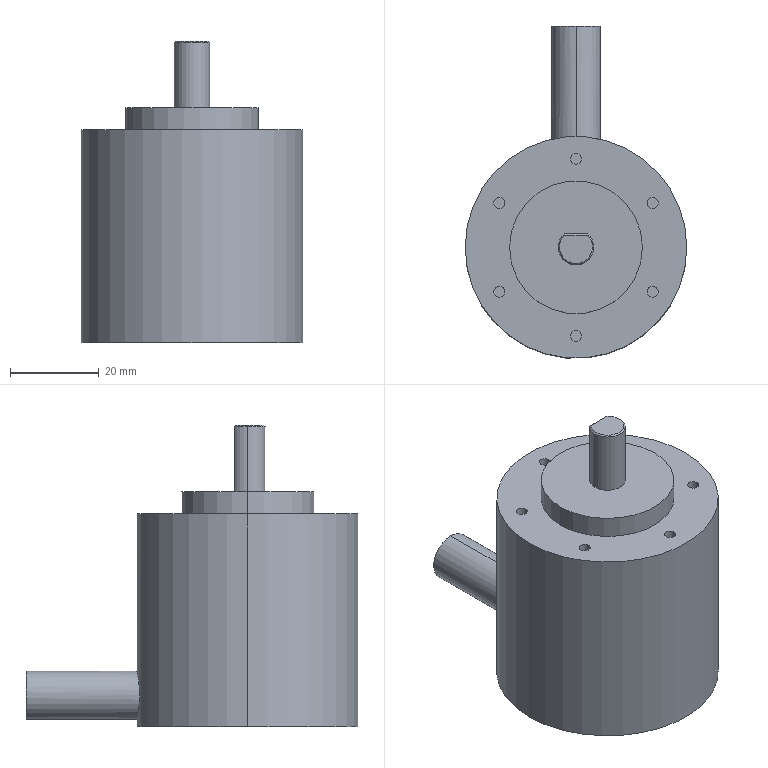Part | SolidWorks | features ICE 4, Chamfer 1, Extrusion 1 | 1 solid | 37 faces | box 50 x 75 x 68 mm | volume 100645 mm3 | cylinder 21 | plane 13 | cone 3 | commonest cylinder face diameters 2.5 x12 8 x3 10.956 x2 30 x2 50 x2
STEP:
#1=CARTESIAN_POINT('',(-1.25,20.,41.));
#2=VERTEX_POINT('',#1);
#3=CARTESIAN_POINT('',(1.25,20.,41.));
#4=VERTEX_POINT('',#3);
#5=CARTESIAN_POINT('',(0.,20.,41.));
#6=DIRECTION('',(0.,0.,1.));
#7=DIRECTION('',(1.,0.,0.));
#8=AXIS2_PLACEMENT_3D('',#5,#6,#7);
#9=CIRCLE('',#8,1.25);
#10=EDGE_CURVE('',#2,#4,#9,.T.);
#11=ORIENTED_EDGE('',*,*,#10,.F.);
#12=CARTESIAN_POINT('',(-1.25,20.,48.));
#13=VERTEX_POINT('',#12);
#14=CARTESIAN_POINT('',(-1.25,20.,41.));
#15=DIRECTION('',(0.,0.,1.));
#16=VECTOR('',#15,1000.);
#17=LINE('',#14,#16);
#18=EDGE_CURVE('',#2,#13,#17,.T.);
#19=ORIENTED_EDGE('',*,*,#18,.T.);
#20=CARTESIAN_POINT('',(1.25,20.,48.));
#21=VERTEX_POINT('',#20);
#22=CARTESIAN_POINT('',(0.,20.,48.));
#23=DIRECTION('',(0.,0.,1.));
#24=DIRECTION('',(1.,0.,0.));
#25=AXIS2_PLACEMENT_3D('',#22,#23,#24);
#26=CIRCLE('',#25,1.25);
#27=EDGE_CURVE('',#13,#21,#26,.T.);
#28=ORIENTED_EDGE('',*,*,#27,.T.);
#29=CARTESIAN_POINT('',(1.25,20.,41.));
#30=DIRECTION('',(0.,0.,1.));
#31=VECTOR('',#30,1000.);
#32=LINE('',#29,#31);
#33=EDGE_CURVE('',#4,#21,#32,.T.);
#34=ORIENTED_EDGE('',*,*,#33,.F.);
#35=EDGE_LOOP('',(#11,#19,#28,#34));
#36=FACE_OUTER_BOUND('',#35,.T.);
#37=CARTESIAN_POINT('',(0.,20.,41.));
#38=DIRECTION('',(0.,0.,1.));
#39=DIRECTION('',(1.,0.,0.));
#40=AXIS2_PLACEMENT_3D('',#37,#38,#39);
#41=CYLINDRICAL_SURFACE('',#40,1.25);
#42=ADVANCED_FACE('',(#36),#41,.F.);
#43=CARTESIAN_POINT('',(-18.571,10.,41.));
#44=VERTEX_POINT('',#43);
#45=CARTESIAN_POINT('',(-16.071,10.,41.));
#46=VERTEX_POINT('',#45);
#47=CARTESIAN_POINT('',(-17.321,10.,41.));
#48=DIRECTION('',(0.,0.,1.));
#49=DIRECTION('',(1.,0.,0.));
#50=AXIS2_PLACEMENT_3D('',#47,#48,#49);
#51=CIRCLE('',#50,1.25);
#52=EDGE_CURVE('',#44,#46,#51,.T.);
#53=ORIENTED_EDGE('',*,*,#52,.F.);
#54=CARTESIAN_POINT('',(-18.571,10.,48.));
#55=VERTEX_POINT('',#54);
#56=CARTESIAN_POINT('',(-18.571,10.,41.));
#57=DIRECTION('',(0.,0.,1.));
#58=VECTOR('',#57,1000.);
#59=LINE('',#56,#58);
#60=EDGE_CURVE('',#44,#55,#59,.T.);
#61=ORIENTED_EDGE('',*,*,#60,.T.);
#62=CARTESIAN_POINT('',(-16.071,10.,48.));
#63=VERTEX_POINT('',#62);
#64=CARTESIAN_POINT('',(-17.321,10.,48.));
#65=DIRECTION('',(0.,0.,1.));
#66=DIRECTION('',(1.,0.,0.));
#67=AXIS2_PLACEMENT_3D('',#64,#65,#66);
#68=CIRCLE('',#67,1.25);
#69=EDGE_CURVE('',#55,#63,#68,.T.);
#70=ORIENTED_EDGE('',*,*,#69,.T.);
#71=CARTESIAN_POINT('',(-16.071,10.,41.));
#72=DIRECTION('',(0.,0.,1.));
#73=VECTOR('',#72,1000.);
#74=LINE('',#71,#73);
#75=EDGE_CURVE('',#46,#63,#74,.T.);
#76=ORIENTED_EDGE('',*,*,#75,.F.);
#77=EDGE_LOOP('',(#53,#61,#70,#76));
#78=FACE_OUTER_BOUND('',#77,.T.);
#79=CARTESIAN_POINT('',(-17.321,10.,41.));
#80=DIRECTION('',(0.,0.,1.));
#81=DIRECTION('',(1.,0.,0.));
#82=AXIS2_PLACEMENT_3D('',#79,#80,#81);
#83=CYLINDRICAL_SURFACE('',#82,1.25);
#84=ADVANCED_FACE('',(#78),#83,.F.);
#85=CARTESIAN_POINT('',(-18.571,-10.,41.));
#86=VERTEX_POINT('',#85);
#87=CARTESIAN_POINT('',(-16.071,-10.,41.));
#88=VERTEX_POINT('',#87);
#89=CARTESIAN_POINT('',(-17.321,-10.,41.));
#90=DIRECTION('',(0.,0.,1.));
#91=DIRECTION('',(1.,0.,0.));
#92=AXIS2_PLACEMENT_3D('',#89,#90,#91);
#93=CIRCLE('',#92,1.25);
#94=EDGE_CURVE('',#86,#88,#93,.T.);
#95=ORIENTED_EDGE('',*,*,#94,.F.);
#96=CARTESIAN_POINT('',(-18.571,-10.,48.));
#97=VERTEX_POINT('',#96);
#98=CARTESIAN_POINT('',(-18.571,-10.,41.));
#99=DIRECTION('',(0.,0.,1.));
#100=VECTOR('',#99,1000.);
#101=LINE('',#98,#100);
#102=EDGE_CURVE('',#86,#97,#101,.T.);
#103=ORIENTED_EDGE('',*,*,#102,.T.);
#104=CARTESIAN_POINT('',(-16.071,-10.,48.));
#105=VERTEX_POINT('',#104);
#106=CARTESIAN_POINT('',(-17.321,-10.,48.));
#107=DIRECTION('',(0.,0.,1.));
#108=DIRECTION('',(1.,0.,0.));
#109=AXIS2_PLACEMENT_3D('',#106,#107,#108);
#110=CIRCLE('',#109,1.25);
#111=EDGE_CURVE('',#97,#105,#110,.T.);
#112=ORIENTED_EDGE('',*,*,#111,.T.);
#113=CARTESIAN_POINT('',(-16.071,-10.,41.));
#114=DIRECTION('',(0.,0.,1.));
#115=VECTOR('',#114,1000.);
#116=LINE('',#113,#115);
#117=EDGE_CURVE('',#88,#105,#116,.T.);
#118=ORIENTED_EDGE('',*,*,#117,.F.);
#119=EDGE_LOOP('',(#95,#103,#112,#118));
#120=FACE_OUTER_BOUND('',#119,.T.);
#121=CARTESIAN_POINT('',(-17.321,-10.,41.));
#122=DIRECTION('',(0.,0.,1.));
#123=DIRECTION('',(1.,0.,0.));
#124=AXIS2_PLACEMENT_3D('',#121,#122,#123);
#125=CYLINDRICAL_SURFACE('',#124,1.25);
#126=ADVANCED_FACE('',(#120),#125,.F.);
#127=CARTESIAN_POINT('',(-1.25,-20.,41.));
#128=VERTEX_POINT('',#127);
#129=CARTESIAN_POINT('',(1.25,-20.,41.));
#130=VERTEX_POINT('',#129);
#131=CARTESIAN_POINT('',(0.,-20.,41.));
#132=DIRECTION('',(0.,0.,1.));
#133=DIRECTION('',(1.,0.,0.));
#134=AXIS2_PLACEMENT_3D('',#131,#132,#133);
#135=CIRCLE('',#134,1.25);
#136=EDGE_CURVE('',#128,#130,#135,.T.);
#137=ORIENTED_EDGE('',*,*,#136,.F.);
#138=CARTESIAN_POINT('',(-1.25,-20.,48.));
#139=VERTEX_POINT('',#138);
#140=CARTESIAN_POINT('',(-1.25,-20.,41.));
#141=DIRECTION('',(0.,0.,1.));
#142=VECTOR('',#141,1000.);
#143=LINE('',#140,#142);
#144=EDGE_CURVE('',#128,#139,#143,.T.);
#145=ORIENTED_EDGE('',*,*,#144,.T.);
#146=CARTESIAN_POINT('',(1.25,-20.,48.));
#147=VERTEX_POINT('',#146);
#148=CARTESIAN_POINT('',(0.,-20.,48.));
#149=DIRECTION('',(0.,0.,1.));
#150=DIRECTION('',(1.,0.,0.));
#151=AXIS2_PLACEMENT_3D('',#148,#149,#150);
#152=CIRCLE('',#151,1.25);
#153=EDGE_CURVE('',#139,#147,#152,.T.);
#154=ORIENTED_EDGE('',*,*,#153,.T.);
#155=CARTESIAN_POINT('',(1.25,-20.,41.));
#156=DIRECTION('',(0.,0.,1.));
#157=VECTOR('',#156,1000.);
#158=LINE('',#155,#157);
#159=EDGE_CURVE('',#130,#147,#158,.T.);
#160=ORIENTED_EDGE('',*,*,#159,.F.);
#161=EDGE_LOOP('',(#137,#145,#154,#160));
#162=FACE_OUTER_BOUND('',#161,.T.);
#163=CARTESIAN_POINT('',(0.,-20.,41.));
#164=DIRECTION('',(0.,0.,1.));
#165=DIRECTION('',(1.,0.,0.));
#166=AXIS2_PLACEMENT_3D('',#163,#164,#165);
#167=CYLINDRICAL_SURFACE('',#166,1.25);
#168=ADVANCED_FACE('',(#162),#167,.F.);
#169=CARTESIAN_POINT('',(16.071,-10.,41.));
#170=VERTEX_POINT('',#169);
#171=CARTESIAN_POINT('',(18.571,-10.,41.));
#172=VERTEX_POINT('',#171);
#173=CARTESIAN_POINT('',(17.321,-10.,41.));
#174=DIRECTION('',(0.,0.,1.));
#175=DIRECTION('',(1.,0.,0.));
#176=AXIS2_PLACEMENT_3D('',#173,#174,#175);
#177=CIRCLE('',#176,1.25);
#178=EDGE_CURVE('',#170,#172,#177,.T.);
#179=ORIENTED_EDGE('',*,*,#178,.F.);
#180=CARTESIAN_POINT('',(16.071,-10.,48.));
#181=VERTEX_POINT('',#180);
#182=CARTESIAN_POINT('',(16.071,-10.,41.));
#183=DIRECTION('',(0.,0.,1.));
#184=VECTOR('',#183,1000.);
#185=LINE('',#182,#184);
#186=EDGE_CURVE('',#170,#181,#185,.T.);
#187=ORIENTED_EDGE('',*,*,#186,.T.);
#188=CARTESIAN_POINT('',(18.571,-10.,48.));
#189=VERTEX_POINT('',#188);
#190=CARTESIAN_POINT('',(17.321,-10.,48.));
#191=DIRECTION('',(0.,0.,1.));
#192=DIRECTION('',(1.,0.,0.));
#193=AXIS2_PLACEMENT_3D('',#190,#191,#192);
#194=CIRCLE('',#193,1.25);
#195=EDGE_CURVE('',#181,#189,#194,.T.);
#196=ORIENTED_EDGE('',*,*,#195,.T.);
#197=CARTESIAN_POINT('',(18.571,-10.,41.));
#198=DIRECTION('',(0.,0.,1.));
#199=VECTOR('',#198,1000.);
#200=LINE('',#197,#199);
#201=EDGE_CURVE('',#172,#189,#200,.T.);
#202=ORIENTED_EDGE('',*,*,#201,.F.);
#203=EDGE_LOOP('',(#179,#187,#196,#202));
#204=FACE_OUTER_BOUND('',#203,.T.);
#205=CARTESIAN_POINT('',(17.321,-10.,41.));
#206=DIRECTION('',(0.,0.,1.));
#207=DIRECTION('',(1.,0.,0.));
#208=AXIS2_PLACEMENT_3D('',#205,#206,#207);
#209=CYLINDRICAL_SURFACE('',#208,1.25);
#210=ADVANCED_FACE('',(#204),#209,.F.);
#211=CARTESIAN_POINT('',(16.071,10.,41.));
#212=VERTEX_POINT('',#211);
#213=CARTESIAN_POINT('',(18.571,10.,41.));
#214=VERTEX_POINT('',#213);
#215=CARTESIAN_POINT('',(17.321,10.,41.));
#216=DIRECTION('',(0.,0.,1.));
#217=DIRECTION('',(1.,0.,0.));
#218=AXIS2_PLACEMENT_3D('',#215,#216,#217);
#219=CIRCLE('',#218,1.25);
#220=EDGE_CURVE('',#212,#214,#219,.T.);
#221=ORIENTED_EDGE('',*,*,#220,.F.);
#222=CARTESIAN_POINT('',(16.071,10.,48.));
#223=VERTEX_POINT('',#222);
#224=CARTESIAN_POINT('',(16.071,10.,41.));
#225=DIRECTION('',(0.,0.,1.));
#226=VECTOR('',#225,1000.);
#227=LINE('',#224,#226);
#228=EDGE_CURVE('',#212,#223,#227,.T.);
#229=ORIENTED_EDGE('',*,*,#228,.T.);
#230=CARTESIAN_POINT('',(18.571,10.,48.));
#231=VERTEX_POINT('',#230);
#232=CARTESIAN_POINT('',(17.321,10.,48.));
#233=DIRECTION('',(0.,0.,1.));
#234=DIRECTION('',(1.,0.,0.));
#235=AXIS2_PLACEMENT_3D('',#232,#233,#234);
#236=CIRCLE('',#235,1.25);
#237=EDGE_CURVE('',#223,#231,#236,.T.);
#238=ORIENTED_EDGE('',*,*,#237,.T.);
#239=CARTESIAN_POINT('',(18.571,10.,41.));
#240=DIRECTION('',(0.,0.,1.));
#241=VECTOR('',#240,1000.);
#242=LINE('',#239,#241);
#243=EDGE_CURVE('',#214,#231,#242,.T.);
#244=ORIENTED_EDGE('',*,*,#243,.F.);
#245=EDGE_LOOP('',(#221,#229,#238,#244));
#246=FACE_OUTER_BOUND('',#245,.T.);
#247=CARTESIAN_POINT('',(17.321,10.,41.));
#248=DIRECTION('',(0.,0.,1.));
#249=DIRECTION('',(1.,0.,0.));
#250=AXIS2_PLACEMENT_3D('',#247,#248,#249);
#251=CYLINDRICAL_SURFACE('',#250,1.25);
#252=ADVANCED_FACE('',(#246),#251,.F.);
#253=CARTESIAN_POINT('',(0.,50.,12.561));
#254=VERTEX_POINT('',#253);
#255=CARTESIAN_POINT('',(0.,50.,1.606));
#256=VERTEX_POINT('',#255);
#257=CARTESIAN_POINT('',(0.,50.,7.083));
#258=DIRECTION('',(0.,1.,0.));
#259=DIRECTION('',(0.,0.,1.));
#260=AXIS2_PLACEMENT_3D('',#257,#258,#259);
#261=CIRCLE('',#260,5.478);
#262=EDGE_CURVE('',#254,#256,#261,.T.);
#263=ORIENTED_EDGE('',*,*,#262,.F.);
#264=CARTESIAN_POINT('',(0.,25.,12.561));
#265=VERTEX_POINT('',#264);
#266=CARTESIAN_POINT('',(0.,50.,12.561));
#267=DIRECTION('',(0.,-1.,0.));
#268=VECTOR('',#267,1000.);
#269=LINE('',#266,#268);
#270=EDGE_CURVE('',#254,#265,#269,.T.);
#271=ORIENTED_EDGE('',*,*,#270,.T.);
#272=CARTESIAN_POINT('',(0.,25.,1.606));
#273=VERTEX_POINT('',#272);
#274=CARTESIAN_POINT('',(0.,25.,12.561));
#275=CARTESIAN_POINT('',(0.358,25.,12.561));
#276=CARTESIAN_POINT('',(0.7147,24.992,12.527));
#277=CARTESIAN_POINT('',(1.425,24.962,12.385));
#278=CARTESIAN_POINT('',(1.769,24.94,12.28));
#279=CARTESIAN_POINT('',(2.263,24.898,12.075));
#280=CARTESIAN_POINT('',(2.425,24.883,11.999));
#281=CARTESIAN_POINT('',(2.742,24.85,11.829));
#282=CARTESIAN_POINT('',(2.897,24.832,11.736));
#283=CARTESIAN_POINT('',(3.344,24.777,11.437));
#284=CARTESIAN_POINT('',(3.619,24.738,11.211));
#285=CARTESIAN_POINT('',(4.124,24.659,10.707));
#286=CARTESIAN_POINT('',(4.355,24.619,10.426));
#287=CARTESIAN_POINT('',(4.751,24.545,9.833));
#288=CARTESIAN_POINT('',(4.92,24.512,9.519));
#289=CARTESIAN_POINT('',(5.127,24.469,9.02));
#290=CARTESIAN_POINT('',(5.189,24.456,8.85));
#291=CARTESIAN_POINT('',(5.293,24.433,8.506));
#292=CARTESIAN_POINT('',(5.337,24.424,8.333));
#293=CARTESIAN_POINT('',(5.442,24.401,7.807));
#294=CARTESIAN_POINT('',(5.478,24.392,7.447));
#295=CARTESIAN_POINT('',(5.478,24.392,6.724));
#296=CARTESIAN_POINT('',(5.443,24.4,6.368));
#297=CARTESIAN_POINT('',(5.303,24.431,5.665));
#298=CARTESIAN_POINT('',(5.197,24.454,5.316));
#299=CARTESIAN_POINT('',(4.923,24.511,4.655));
#300=CARTESIAN_POINT('',(4.755,24.544,4.34));
#301=CARTESIAN_POINT('',(4.456,24.6,3.893));
#302=CARTESIAN_POINT('',(4.348,24.619,3.747));
#303=CARTESIAN_POINT('',(4.121,24.658,3.47));
#304=CARTESIAN_POINT('',(4.002,24.678,3.338));
#305=CARTESIAN_POINT('',(3.624,24.737,2.961));
#306=CARTESIAN_POINT('',(3.348,24.777,2.733));
#307=CARTESIAN_POINT('',(2.749,24.85,2.332));
#308=CARTESIAN_POINT('',(2.435,24.883,2.163));
#309=CARTESIAN_POINT('',(1.776,24.939,1.889));
#310=CARTESIAN_POINT('',(1.428,24.962,1.783));
#311=CARTESIAN_POINT('',(0.7212,24.992,1.641));
#312=CARTESIAN_POINT('',(0.363,25.,1.606));
#313=CARTESIAN_POINT('',(0.,25.,1.606));
#314=B_SPLINE_CURVE_WITH_KNOTS('',3,(#274,#275,#276,#277,#278,#279,#280,#281,#282,#283,#284,#285,#286,#287,#288,#289,#290,#291,#292,#293,#294,#295,#296,#297,#298,#299,#300,#301,#302,#303,#304,#305,#306,#307,#308,#309,#310,#311,#312,#313),.UNSPECIFIED.,.F.,.F.,(4,2,2,2,2,2,2,2,2,2,2,2,2,2,2,2,2,2,2,4),(0.01718,0.01825,0.01933,0.01986,0.0204,0.02147,0.02255,0.02362,0.02416,0.02469,0.02577,0.02684,0.02791,0.02899,0.02952,0.03006,0.03113,0.03221,0.03328,0.03435),.UNSPECIFIED.);
#315=EDGE_CURVE('',#265,#273,#314,.T.);
#316=ORIENTED_EDGE('',*,*,#315,.T.);
#317=CARTESIAN_POINT('',(0.,50.,1.606));
#318=DIRECTION('',(0.,-1.,0.));
#319=VECTOR('',#318,1000.);
#320=LINE('',#317,#319);
#321=EDGE_CURVE('',#256,#273,#320,.T.);
#322=ORIENTED_EDGE('',*,*,#321,.F.);
#323=EDGE_LOOP('',(#263,#271,#316,#322));
#324=FACE_OUTER_BOUND('',#323,.T.);
#325=CARTESIAN_POINT('',(0.,50.,7.083));
#326=DIRECTION('',(0.,-1.,0.));
#327=DIRECTION('',(0.,0.,-1.));
#328=AXIS2_PLACEMENT_3D('',#325,#326,#327);
#329=CYLINDRICAL_SURFACE('',#328,5.478);
#330=ADVANCED_FACE('',(#324),#329,.T.);
#331=CARTESIAN_POINT('',(3.7,0.,68.));
#332=VERTEX_POINT('',#331);
#333=CARTESIAN_POINT('',(2.53,2.7,68.));
#334=VERTEX_POINT('',#333);
#335=CARTESIAN_POINT('',(0.,0.,68.));
#336=DIRECTION('',(0.,0.,1.));
#337=DIRECTION('',(1.,0.,0.));
#338=AXIS2_PLACEMENT_3D('',#335,#336,#337);
#339=CIRCLE('',#338,3.7);
#340=EDGE_CURVE('',#332,#334,#339,.T.);
#341=ORIENTED_EDGE('',*,*,#340,.F.);
#342=CARTESIAN_POINT('',(4.,0.,67.7));
#343=VERTEX_POINT('',#342);
#344=CARTESIAN_POINT('',(3.7,0.,68.));
#345=DIRECTION('',(0.7071,0.,-0.7071));
#346=VECTOR('',#345,1000.);
#347=LINE('',#344,#346);
#348=EDGE_CURVE('',#332,#343,#347,.T.);
#349=ORIENTED_EDGE('',*,*,#348,.T.);
#350=CARTESIAN_POINT('',(2.646,3.,67.7));
#351=VERTEX_POINT('',#350);
#352=CARTESIAN_POINT('',(0.,0.,67.7));
#353=DIRECTION('',(0.,0.,-1.));
#354=DIRECTION('',(1.,0.,0.));
#355=AXIS2_PLACEMENT_3D('',#352,#353,#354);
#356=CIRCLE('',#355,4.);
#357=EDGE_CURVE('',#351,#343,#356,.T.);
#358=ORIENTED_EDGE('',*,*,#357,.F.);
#359=CARTESIAN_POINT('',(2.53,2.7,68.));
#360=CARTESIAN_POINT('',(2.569,2.8,67.9));
#361=CARTESIAN_POINT('',(2.608,2.9,67.8));
#362=CARTESIAN_POINT('',(2.646,3.,67.7));
#363=B_SPLINE_CURVE_WITH_KNOTS('',3,(#359,#360,#361,#362),.UNSPECIFIED.,.F.,.F.,(4,4),(0.,0.0004398),.UNSPECIFIED.);
#364=EDGE_CURVE('',#334,#351,#363,.T.);
#365=ORIENTED_EDGE('',*,*,#364,.F.);
#366=EDGE_LOOP('',(#341,#349,#358,#365));
#367=FACE_OUTER_BOUND('',#366,.T.);
#368=CARTESIAN_POINT('',(0.,0.,68.));
#369=DIRECTION('',(0.,0.,-1.));
#370=DIRECTION('',(-1.,0.,0.));
#371=AXIS2_PLACEMENT_3D('',#368,#369,#370);
#372=CONICAL_SURFACE('',#371,3.7,0.7854);
#373=ADVANCED_FACE('',(#367),#372,.T.);
#374=ORIENTED_EDGE('',*,*,#348,.F.);
#375=CARTESIAN_POINT('',(-3.7,0.,68.));
#376=VERTEX_POINT('',#375);
#377=CARTESIAN_POINT('',(0.,0.,68.));
#378=DIRECTION('',(0.,0.,1.));
#379=DIRECTION('',(1.,0.,0.));
#380=AXIS2_PLACEMENT_3D('',#377,#378,#379);
#381=CIRCLE('',#380,3.7);
#382=EDGE_CURVE('',#376,#332,#381,.T.);
#383=ORIENTED_EDGE('',*,*,#382,.F.);
#384=CARTESIAN_POINT('',(-4.,0.,67.7));
#385=VERTEX_POINT('',#384);
#386=CARTESIAN_POINT('',(-3.7,0.,68.));
#387=DIRECTION('',(-0.7071,0.,-0.7071));
#388=VECTOR('',#387,1000.);
#389=LINE('',#386,#388);
#390=EDGE_CURVE('',#376,#385,#389,.T.);
#391=ORIENTED_EDGE('',*,*,#390,.T.);
#392=CARTESIAN_POINT('',(0.,0.,67.7));
#393=DIRECTION('',(0.,0.,-1.));
#394=DIRECTION('',(1.,0.,0.));
#395=AXIS2_PLACEMENT_3D('',#392,#393,#394);
#396=CIRCLE('',#395,4.);
#397=EDGE_CURVE('',#343,#385,#396,.T.);
#398=ORIENTED_EDGE('',*,*,#397,.F.);
#399=EDGE_LOOP('',(#374,#383,#391,#398));
#400=FACE_OUTER_BOUND('',#399,.T.);
#401=CARTESIAN_POINT('',(0.,0.,68.));
#402=DIRECTION('',(0.,0.,-1.));
#403=DIRECTION('',(-1.,0.,0.));
#404=AXIS2_PLACEMENT_3D('',#401,#402,#403);
#405=CONICAL_SURFACE('',#404,3.7,0.7854);
#406=ADVANCED_FACE('',(#400),#405,.T.);
#407=ORIENTED_EDGE('',*,*,#357,.T.);
#408=CARTESIAN_POINT('',(4.,0.,53.));
#409=VERTEX_POINT('',#408);
#410=CARTESIAN_POINT('',(4.,0.,68.));
#411=DIRECTION('',(0.,0.,-1.));
#412=VECTOR('',#411,1000.);
#413=LINE('',#410,#412);
#414=EDGE_CURVE('',#343,#409,#413,.T.);
#415=ORIENTED_EDGE('',*,*,#414,.T.);
#416=CARTESIAN_POINT('',(2.646,3.,53.));
#417=VERTEX_POINT('',#416);
#418=CARTESIAN_POINT('',(0.,0.,53.));
#419=DIRECTION('',(0.,0.,1.));
#420=DIRECTION('',(1.,0.,0.));
#421=AXIS2_PLACEMENT_3D('',#418,#419,#420);
#422=CIRCLE('',#421,4.);
#423=EDGE_CURVE('',#409,#417,#422,.T.);
#424=ORIENTED_EDGE('',*,*,#423,.T.);
#425=CARTESIAN_POINT('',(2.646,3.,68.));
#426=DIRECTION('',(0.,0.,-1.));
#427=VECTOR('',#426,1000.);
#428=LINE('',#425,#427);
#429=EDGE_CURVE('',#351,#417,#428,.T.);
#430=ORIENTED_EDGE('',*,*,#429,.F.);
#431=EDGE_LOOP('',(#407,#415,#424,#430));
#432=FACE_OUTER_BOUND('',#431,.T.);
#433=CARTESIAN_POINT('',(0.,0.,68.));
#434=DIRECTION('',(0.,0.,-1.));
#435=DIRECTION('',(-1.,0.,0.));
#436=AXIS2_PLACEMENT_3D('',#433,#434,#435);
#437=CYLINDRICAL_SURFACE('',#436,4.);
#438=ADVANCED_FACE('',(#432),#437,.T.);
#439=ORIENTED_EDGE('',*,*,#414,.F.);
#440=ORIENTED_EDGE('',*,*,#397,.T.);
#441=CARTESIAN_POINT('',(-4.,0.,53.));
#442=VERTEX_POINT('',#441);
#443=CARTESIAN_POINT('',(-4.,0.,68.));
#444=DIRECTION('',(0.,0.,-1.));
#445=VECTOR('',#444,1000.);
#446=LINE('',#443,#445);
#447=EDGE_CURVE('',#385,#442,#446,.T.);
#448=ORIENTED_EDGE('',*,*,#447,.T.);
#449=CARTESIAN_POINT('',(0.,0.,53.));
#450=DIRECTION('',(0.,0.,1.));
#451=DIRECTION('',(1.,0.,0.));
#452=AXIS2_PLACEMENT_3D('',#449,#450,#451);
#453=CIRCLE('',#452,4.);
#454=EDGE_CURVE('',#442,#409,#453,.T.);
#455=ORIENTED_EDGE('',*,*,#454,.T.);
#456=EDGE_LOOP('',(#439,#440,#448,#455));
#457=FACE_OUTER_BOUND('',#456,.T.);
#458=CARTESIAN_POINT('',(0.,0.,68.));
#459=DIRECTION('',(0.,0.,-1.));
#460=DIRECTION('',(-1.,0.,0.));
#461=AXIS2_PLACEMENT_3D('',#458,#459,#460);
#462=CYLINDRICAL_SURFACE('',#461,4.);
#463=ADVANCED_FACE('',(#457),#462,.T.);
#464=CARTESIAN_POINT('',(15.,0.,53.));
#465=VERTEX_POINT('',#464);
#466=CARTESIAN_POINT('',(-15.,0.,53.));
#467=VERTEX_POINT('',#466);
#468=CARTESIAN_POINT('',(0.,0.,53.));
#469=DIRECTION('',(0.,0.,1.));
#470=DIRECTION('',(1.,0.,0.));
#471=AXIS2_PLACEMENT_3D('',#468,#469,#470);
#472=CIRCLE('',#471,15.);
#473=EDGE_CURVE('',#465,#467,#472,.T.);
#474=ORIENTED_EDGE('',*,*,#473,.F.);
#475=CARTESIAN_POINT('',(15.,0.,48.));
#476=VERTEX_POINT('',#475);
#477=CARTESIAN_POINT('',(15.,0.,53.));
#478=DIRECTION('',(0.,0.,-1.));
#479=VECTOR('',#478,1000.);
#480=LINE('',#477,#479);
#481=EDGE_CURVE('',#465,#476,#480,.T.);
#482=ORIENTED_EDGE('',*,*,#481,.T.);
#483=CARTESIAN_POINT('',(-15.,0.,48.));
#484=VERTEX_POINT('',#483);
#485=CARTESIAN_POINT('',(0.,0.,48.));
#486=DIRECTION('',(0.,0.,1.));
#487=DIRECTION('',(1.,0.,0.));
#488=AXIS2_PLACEMENT_3D('',#485,#486,#487);
#489=CIRCLE('',#488,15.);
#490=EDGE_CURVE('',#476,#484,#489,.T.);
#491=ORIENTED_EDGE('',*,*,#490,.T.);
#492=CARTESIAN_POINT('',(-15.,0.,53.));
#493=DIRECTION('',(0.,0.,-1.));
#494=VECTOR('',#493,1000.);
#495=LINE('',#492,#494);
#496=EDGE_CURVE('',#467,#484,#495,.T.);
#497=ORIENTED_EDGE('',*,*,#496,.F.);
#498=EDGE_LOOP('',(#474,#482,#491,#497));
#499=FACE_OUTER_BOUND('',#498,.T.);
#500=CARTESIAN_POINT('',(0.,0.,53.));
#501=DIRECTION('',(0.,0.,-1.));
#502=DIRECTION('',(-1.,0.,0.));
#503=AXIS2_PLACEMENT_3D('',#500,#501,#502);
#504=CYLINDRICAL_SURFACE('',#503,15.);
#505=ADVANCED_FACE('',(#499),#504,.T.);
#506=CARTESIAN_POINT('',(0.,25.,1.606));
#507=CARTESIAN_POINT('',(-0.3631,25.,1.606));
#508=CARTESIAN_POINT('',(-0.72,24.992,1.641));
#509=CARTESIAN_POINT('',(-1.246,24.97,1.746));
#510=CARTESIAN_POINT('',(-1.42,24.96,1.79));
#511=CARTESIAN_POINT('',(-1.765,24.938,1.895));
#512=CARTESIAN_POINT('',(-1.936,24.925,1.956));
#513=CARTESIAN_POINT('',(-2.433,24.884,2.162));
#514=CARTESIAN_POINT('',(-2.747,24.85,2.331));
#515=CARTESIAN_POINT('',(-3.342,24.777,2.728));
#516=CARTESIAN_POINT('',(-3.623,24.737,2.959));
#517=CARTESIAN_POINT('',(-4.126,24.658,3.463));
#518=CARTESIAN_POINT('',(-4.353,24.619,3.738));
#519=CARTESIAN_POINT('',(-4.753,24.545,4.337));
#520=CARTESIAN_POINT('',(-4.923,24.511,4.654));
#521=CARTESIAN_POINT('',(-5.128,24.469,5.148));
#522=CARTESIAN_POINT('',(-5.188,24.456,5.316));
#523=CARTESIAN_POINT('',(-5.293,24.433,5.659));
#524=CARTESIAN_POINT('',(-5.337,24.424,5.836));
#525=CARTESIAN_POINT('',(-5.443,24.4,6.367));
#526=CARTESIAN_POINT('',(-5.478,24.392,6.723));
#527=CARTESIAN_POINT('',(-5.478,24.392,7.44));
#528=CARTESIAN_POINT('',(-5.442,24.401,7.804));
#529=CARTESIAN_POINT('',(-5.302,24.431,8.508));
#530=CARTESIAN_POINT('',(-5.198,24.454,8.85));
#531=CARTESIAN_POINT('',(-4.991,24.497,9.348));
#532=CARTESIAN_POINT('',(-4.913,24.513,9.512));
#533=CARTESIAN_POINT('',(-4.744,24.546,9.828));
#534=CARTESIAN_POINT('',(-4.652,24.564,9.981));
#535=CARTESIAN_POINT('',(-4.355,24.619,10.425));
#536=CARTESIAN_POINT('',(-4.127,24.658,10.703));
#537=CARTESIAN_POINT('',(-3.619,24.738,11.212));
#538=CARTESIAN_POINT('',(-3.343,24.777,11.438));
#539=CARTESIAN_POINT('',(-2.751,24.85,11.834));
#540=CARTESIAN_POINT('',(-2.43,24.884,12.006));
#541=CARTESIAN_POINT('',(-1.768,24.94,12.281));
#542=CARTESIAN_POINT('',(-1.426,24.962,12.385));
#543=CARTESIAN_POINT('',(-0.898,24.984,12.49));
#544=CARTESIAN_POINT('',(-0.718,24.99,12.517));
#545=CARTESIAN_POINT('',(-0.3585,24.998,12.553));
#546=CARTESIAN_POINT('',(-0.1791,25.,12.561));
#547=CARTESIAN_POINT('',(0.,25.,12.561));
#548=B_SPLINE_CURVE_WITH_KNOTS('',3,(#506,#507,#508,#509,#510,#511,#512,#513,#514,#515,#516,#517,#518,#519,#520,#521,#522,#523,#524,#525,#526,#527,#528,#529,#530,#531,#532,#533,#534,#535,#536,#537,#538,#539,#540,#541,#542,#543,#544,#545,#546,#547),.UNSPECIFIED.,.F.,.F.,(4,2,2,2,2,2,2,2,2,2,2,2,2,2,2,2,2,2,2,2,4),(0.,0.001074,0.001611,0.002147,0.003221,0.004295,0.005368,0.006442,0.006979,0.007516,0.008589,0.009663,0.01074,0.01127,0.01181,0.01288,0.01396,0.01503,0.01611,0.01664,0.01718),.UNSPECIFIED.);
#549=EDGE_CURVE('',#273,#265,#548,.T.);
#550=ORIENTED_EDGE('',*,*,#549,.F.);
#551=ORIENTED_EDGE('',*,*,#315,.F.);
#552=EDGE_LOOP('',(#550,#551));
#553=FACE_BOUND('',#552,.T.);
#554=CARTESIAN_POINT('',(25.,0.,48.));
#555=VERTEX_POINT('',#554);
#556=CARTESIAN_POINT('',(-25.,0.,48.));
#557=VERTEX_POINT('',#556);
#558=CARTESIAN_POINT('',(0.,0.,48.));
#559=DIRECTION('',(0.,0.,1.));
#560=DIRECTION('',(1.,0.,0.));
#561=AXIS2_PLACEMENT_3D('',#558,#559,#560);
#562=CIRCLE('',#561,25.);
#563=EDGE_CURVE('',#555,#557,#562,.T.);
#564=ORIENTED_EDGE('',*,*,#563,.F.);
#565=CARTESIAN_POINT('',(25.,0.,0.));
#566=VERTEX_POINT('',#565);
#567=CARTESIAN_POINT('',(25.,0.,48.));
#568=DIRECTION('',(0.,0.,-1.));
#569=VECTOR('',#568,1000.);
#570=LINE('',#567,#569);
#571=EDGE_CURVE('',#555,#566,#570,.T.);
#572=ORIENTED_EDGE('',*,*,#571,.T.);
#573=CARTESIAN_POINT('',(-25.,0.,0.));
#574=VERTEX_POINT('',#573);
#575=CARTESIAN_POINT('',(0.,0.,0.));
#576=DIRECTION('',(0.,0.,1.));
#577=DIRECTION('',(1.,0.,0.));
#578=AXIS2_PLACEMENT_3D('',#575,#576,#577);
#579=CIRCLE('',#578,25.);
#580=EDGE_CURVE('',#566,#574,#579,.T.);
#581=ORIENTED_EDGE('',*,*,#580,.T.);
#582=CARTESIAN_POINT('',(-25.,0.,48.));
#583=DIRECTION('',(0.,0.,-1.));
#584=VECTOR('',#583,1000.);
#585=LINE('',#582,#584);
#586=EDGE_CURVE('',#557,#574,#585,.T.);
#587=ORIENTED_EDGE('',*,*,#586,.F.);
#588=EDGE_LOOP('',(#564,#572,#581,#587));
#589=FACE_OUTER_BOUND('',#588,.T.);
#590=CARTESIAN_POINT('',(0.,0.,48.));
#591=DIRECTION('',(0.,0.,-1.));
#592=DIRECTION('',(-1.,0.,0.));
#593=AXIS2_PLACEMENT_3D('',#590,#591,#592);
#594=CYLINDRICAL_SURFACE('',#593,25.);
#595=ADVANCED_FACE('',(#553,#589),#594,.T.);
#596=ORIENTED_EDGE('',*,*,#571,.F.);
#597=CARTESIAN_POINT('',(0.,0.,48.));
#598=DIRECTION('',(0.,0.,1.));
#599=DIRECTION('',(1.,0.,0.));
#600=AXIS2_PLACEMENT_3D('',#597,#598,#599);
#601=CIRCLE('',#600,25.);
#602=EDGE_CURVE('',#557,#555,#601,.T.);
#603=ORIENTED_EDGE('',*,*,#602,.F.);
#604=ORIENTED_EDGE('',*,*,#586,.T.);
#605=CARTESIAN_POINT('',(0.,0.,0.));
#606=DIRECTION('',(0.,0.,1.));
#607=DIRECTION('',(1.,0.,0.));
#608=AXIS2_PLACEMENT_3D('',#605,#606,#607);
#609=CIRCLE('',#608,25.);
#610=EDGE_CURVE('',#574,#566,#609,.T.);
#611=ORIENTED_EDGE('',*,*,#610,.T.);
#612=EDGE_LOOP('',(#596,#603,#604,#611));
#613=FACE_OUTER_BOUND('',#612,.T.);
#614=CARTESIAN_POINT('',(0.,0.,48.));
#615=DIRECTION('',(0.,0.,-1.));
#616=DIRECTION('',(-1.,0.,0.));
#617=AXIS2_PLACEMENT_3D('',#614,#615,#616);
#618=CYLINDRICAL_SURFACE('',#617,25.);
#619=ADVANCED_FACE('',(#613),#618,.T.);
#620=CARTESIAN_POINT('',(0.,20.,48.));
#621=DIRECTION('',(0.,0.,1.));
#622=DIRECTION('',(1.,0.,0.));
#623=AXIS2_PLACEMENT_3D('',#620,#621,#622);
#624=CIRCLE('',#623,1.25);
#625=EDGE_CURVE('',#21,#13,#624,.T.);
#626=ORIENTED_EDGE('',*,*,#625,.F.);
#627=ORIENTED_EDGE('',*,*,#27,.F.);
#628=EDGE_LOOP('',(#626,#627));
#629=FACE_BOUND('',#628,.T.);
#630=CARTESIAN_POINT('',(-17.321,10.,48.));
#631=DIRECTION('',(0.,0.,1.));
#632=DIRECTION('',(1.,0.,0.));
#633=AXIS2_PLACEMENT_3D('',#630,#631,#632);
#634=CIRCLE('',#633,1.25);
#635=EDGE_CURVE('',#63,#55,#634,.T.);
#636=ORIENTED_EDGE('',*,*,#635,.F.);
#637=ORIENTED_EDGE('',*,*,#69,.F.);
#638=EDGE_LOOP('',(#636,#637));
#639=FACE_BOUND('',#638,.T.);
#640=CARTESIAN_POINT('',(-17.321,-10.,48.));
#641=DIRECTION('',(0.,0.,1.));
#642=DIRECTION('',(1.,0.,0.));
#643=AXIS2_PLACEMENT_3D('',#640,#641,#642);
#644=CIRCLE('',#643,1.25);
#645=EDGE_CURVE('',#105,#97,#644,.T.);
#646=ORIENTED_EDGE('',*,*,#645,.F.);
#647=ORIENTED_EDGE('',*,*,#111,.F.);
#648=EDGE_LOOP('',(#646,#647));
#649=FACE_BOUND('',#648,.T.);
#650=CARTESIAN_POINT('',(0.,-20.,48.));
#651=DIRECTION('',(0.,0.,1.));
#652=DIRECTION('',(1.,0.,0.));
#653=AXIS2_PLACEMENT_3D('',#650,#651,#652);
#654=CIRCLE('',#653,1.25);
#655=EDGE_CURVE('',#147,#139,#654,.T.);
#656=ORIENTED_EDGE('',*,*,#655,.F.);
#657=ORIENTED_EDGE('',*,*,#153,.F.);
#658=EDGE_LOOP('',(#656,#657));
#659=FACE_BOUND('',#658,.T.);
#660=CARTESIAN_POINT('',(17.321,-10.,48.));
#661=DIRECTION('',(0.,0.,1.));
#662=DIRECTION('',(1.,0.,0.));
#663=AXIS2_PLACEMENT_3D('',#660,#661,#662);
#664=CIRCLE('',#663,1.25);
#665=EDGE_CURVE('',#189,#181,#664,.T.);
#666=ORIENTED_EDGE('',*,*,#665,.F.);
#667=ORIENTED_EDGE('',*,*,#195,.F.);
#668=EDGE_LOOP('',(#666,#667));
#669=FACE_BOUND('',#668,.T.);
#670=CARTESIAN_POINT('',(17.321,10.,48.));
#671=DIRECTION('',(0.,0.,1.));
#672=DIRECTION('',(1.,0.,0.));
#673=AXIS2_PLACEMENT_3D('',#670,#671,#672);
#674=CIRCLE('',#673,1.25);
#675=EDGE_CURVE('',#231,#223,#674,.T.);
#676=ORIENTED_EDGE('',*,*,#675,.F.);
#677=ORIENTED_EDGE('',*,*,#237,.F.);
#678=EDGE_LOOP('',(#676,#677));
#679=FACE_BOUND('',#678,.T.);
#680=CARTESIAN_POINT('',(0.,0.,48.));
#681=DIRECTION('',(0.,0.,1.));
#682=DIRECTION('',(1.,0.,0.));
#683=AXIS2_PLACEMENT_3D('',#680,#681,#682);
#684=CIRCLE('',#683,15.);
#685=EDGE_CURVE('',#484,#476,#684,.T.);
#686=ORIENTED_EDGE('',*,*,#685,.F.);
#687=ORIENTED_EDGE('',*,*,#490,.F.);
#688=EDGE_LOOP('',(#686,#687));
#689=FACE_BOUND('',#688,.T.);
#690=ORIENTED_EDGE('',*,*,#602,.T.);
#691=ORIENTED_EDGE('',*,*,#563,.T.);
#692=EDGE_LOOP('',(#690,#691));
#693=FACE_OUTER_BOUND('',#692,.T.);
#694=CARTESIAN_POINT('',(0.,0.,48.));
#695=DIRECTION('',(0.,0.,1.));
#696=DIRECTION('',(1.,0.,0.));
#697=AXIS2_PLACEMENT_3D('',#694,#695,#696);
#698=PLANE('',#697);
#699=ADVANCED_FACE('',(#629,#639,#649,#659,#669,#679,#689,#693),#698,.T.);
#700=ORIENTED_EDGE('',*,*,#610,.F.);
#701=ORIENTED_EDGE('',*,*,#580,.F.);
#702=EDGE_LOOP('',(#700,#701));
#703=FACE_OUTER_BOUND('',#702,.T.);
#704=CARTESIAN_POINT('',(0.,0.,0.));
#705=DIRECTION('',(0.,0.,1.));
#706=DIRECTION('',(1.,0.,0.));
#707=AXIS2_PLACEMENT_3D('',#704,#705,#706);
#708=PLANE('',#707);
#709=ADVANCED_FACE('',(#703),#708,.F.);
#710=ORIENTED_EDGE('',*,*,#481,.F.);
#711=CARTESIAN_POINT('',(0.,0.,53.));
#712=DIRECTION('',(0.,0.,1.));
#713=DIRECTION('',(1.,0.,0.));
#714=AXIS2_PLACEMENT_3D('',#711,#712,#713);
#715=CIRCLE('',#714,15.);
#716=EDGE_CURVE('',#467,#465,#715,.T.);
#717=ORIENTED_EDGE('',*,*,#716,.F.);
#718=ORIENTED_EDGE('',*,*,#496,.T.);
#719=ORIENTED_EDGE('',*,*,#685,.T.);
#720=EDGE_LOOP('',(#710,#717,#718,#719));
#721=FACE_OUTER_BOUND('',#720,.T.);
#722=CARTESIAN_POINT('',(0.,0.,53.));
#723=DIRECTION('',(0.,0.,-1.));
#724=DIRECTION('',(-1.,0.,0.));
#725=AXIS2_PLACEMENT_3D('',#722,#723,#724);
#726=CYLINDRICAL_SURFACE('',#725,15.);
#727=ADVANCED_FACE('',(#721),#726,.T.);
#728=CARTESIAN_POINT('',(-2.646,3.,53.));
#729=VERTEX_POINT('',#728);
#730=CARTESIAN_POINT('',(0.,0.,53.));
#731=DIRECTION('',(0.,0.,1.));
#732=DIRECTION('',(1.,0.,0.));
#733=AXIS2_PLACEMENT_3D('',#730,#731,#732);
#734=CIRCLE('',#733,4.);
#735=EDGE_CURVE('',#729,#442,#734,.T.);
#736=ORIENTED_EDGE('',*,*,#735,.F.);
#737=CARTESIAN_POINT('',(-2.646,3.,53.));
#738=DIRECTION('',(-1.,0.,0.));
#739=VECTOR('',#738,1000.);
#740=LINE('',#737,#739);
#741=EDGE_CURVE('',#417,#729,#740,.T.);
#742=ORIENTED_EDGE('',*,*,#741,.F.);
#743=ORIENTED_EDGE('',*,*,#423,.F.);
#744=ORIENTED_EDGE('',*,*,#454,.F.);
#745=EDGE_LOOP('',(#736,#742,#743,#744));
#746=FACE_BOUND('',#745,.T.);
#747=ORIENTED_EDGE('',*,*,#716,.T.);
#748=ORIENTED_EDGE('',*,*,#473,.T.);
#749=EDGE_LOOP('',(#747,#748));
#750=FACE_OUTER_BOUND('',#749,.T.);
#751=CARTESIAN_POINT('',(0.,0.,53.));
#752=DIRECTION('',(0.,0.,1.));
#753=DIRECTION('',(1.,0.,0.));
#754=AXIS2_PLACEMENT_3D('',#751,#752,#753);
#755=PLANE('',#754);
#756=ADVANCED_FACE('',(#746,#750),#755,.T.);
#757=ORIENTED_EDGE('',*,*,#447,.F.);
#758=CARTESIAN_POINT('',(-2.646,3.,67.7));
#759=VERTEX_POINT('',#758);
#760=CARTESIAN_POINT('',(0.,0.,67.7));
#761=DIRECTION('',(0.,0.,-1.));
#762=DIRECTION('',(1.,0.,0.));
#763=AXIS2_PLACEMENT_3D('',#760,#761,#762);
#764=CIRCLE('',#763,4.);
#765=EDGE_CURVE('',#385,#759,#764,.T.);
#766=ORIENTED_EDGE('',*,*,#765,.T.);
#767=CARTESIAN_POINT('',(-2.646,3.,68.));
#768=DIRECTION('',(0.,0.,-1.));
#769=VECTOR('',#768,1000.);
#770=LINE('',#767,#769);
#771=EDGE_CURVE('',#759,#729,#770,.T.);
#772=ORIENTED_EDGE('',*,*,#771,.T.);
#773=ORIENTED_EDGE('',*,*,#735,.T.);
#774=EDGE_LOOP('',(#757,#766,#772,#773));
#775=FACE_OUTER_BOUND('',#774,.T.);
#776=CARTESIAN_POINT('',(0.,0.,68.));
#777=DIRECTION('',(0.,0.,-1.));
#778=DIRECTION('',(-1.,0.,0.));
#779=AXIS2_PLACEMENT_3D('',#776,#777,#778);
#780=CYLINDRICAL_SURFACE('',#779,4.);
#781=ADVANCED_FACE('',(#775),#780,.T.);
#782=ORIENTED_EDGE('',*,*,#771,.F.);
#783=CARTESIAN_POINT('',(2.646,3.,67.7));
#784=DIRECTION('',(1.,0.,0.));
#785=VECTOR('',#784,1000.);
#786=LINE('',#783,#785);
#787=EDGE_CURVE('',#759,#351,#786,.T.);
#788=ORIENTED_EDGE('',*,*,#787,.T.);
#789=ORIENTED_EDGE('',*,*,#429,.T.);
#790=ORIENTED_EDGE('',*,*,#741,.T.);
#791=EDGE_LOOP('',(#782,#788,#789,#790));
#792=FACE_OUTER_BOUND('',#791,.T.);
#793=CARTESIAN_POINT('',(-2.646,3.,68.));
#794=DIRECTION('',(0.,-1.,0.));
#795=DIRECTION('',(0.,0.,-1.));
#796=AXIS2_PLACEMENT_3D('',#793,#794,#795);
#797=PLANE('',#796);
#798=ADVANCED_FACE('',(#792),#797,.F.);
#799=CARTESIAN_POINT('',(-2.53,2.7,68.));
#800=VERTEX_POINT('',#799);
#801=CARTESIAN_POINT('',(0.,0.,68.));
#802=DIRECTION('',(0.,0.,1.));
#803=DIRECTION('',(1.,0.,0.));
#804=AXIS2_PLACEMENT_3D('',#801,#802,#803);
#805=CIRCLE('',#804,3.7);
#806=EDGE_CURVE('',#800,#376,#805,.T.);
#807=ORIENTED_EDGE('',*,*,#806,.T.);
#808=ORIENTED_EDGE('',*,*,#382,.T.);
#809=ORIENTED_EDGE('',*,*,#340,.T.);
#810=CARTESIAN_POINT('',(-2.646,2.7,68.));
#811=DIRECTION('',(-1.,0.,0.));
#812=VECTOR('',#811,1000.);
#813=LINE('',#810,#812);
#814=EDGE_CURVE('',#334,#800,#813,.T.);
#815=ORIENTED_EDGE('',*,*,#814,.T.);
#816=EDGE_LOOP('',(#807,#808,#809,#815));
#817=FACE_OUTER_BOUND('',#816,.T.);
#818=CARTESIAN_POINT('',(0.,0.,68.));
#819=DIRECTION('',(0.,0.,1.));
#820=DIRECTION('',(1.,0.,0.));
#821=AXIS2_PLACEMENT_3D('',#818,#819,#820);
#822=PLANE('',#821);
#823=ADVANCED_FACE('',(#817),#822,.T.);
#824=ORIENTED_EDGE('',*,*,#390,.F.);
#825=ORIENTED_EDGE('',*,*,#806,.F.);
#826=CARTESIAN_POINT('',(-2.646,3.,67.7));
#827=CARTESIAN_POINT('',(-2.608,2.9,67.8));
#828=CARTESIAN_POINT('',(-2.569,2.8,67.9));
#829=CARTESIAN_POINT('',(-2.53,2.7,68.));
#830=B_SPLINE_CURVE_WITH_KNOTS('',3,(#826,#827,#828,#829),.UNSPECIFIED.,.F.,.F.,(4,4),(0.,0.0004398),.UNSPECIFIED.);
#831=EDGE_CURVE('',#759,#800,#830,.T.);
#832=ORIENTED_EDGE('',*,*,#831,.F.);
#833=ORIENTED_EDGE('',*,*,#765,.F.);
#834=EDGE_LOOP('',(#824,#825,#832,#833));
#835=FACE_OUTER_BOUND('',#834,.T.);
#836=CARTESIAN_POINT('',(0.,0.,68.));
#837=DIRECTION('',(0.,0.,-1.));
#838=DIRECTION('',(-1.,0.,0.));
#839=AXIS2_PLACEMENT_3D('',#836,#837,#838);
#840=CONICAL_SURFACE('',#839,3.7,0.7854);
#841=ADVANCED_FACE('',(#835),#840,.T.);
#842=ORIENTED_EDGE('',*,*,#364,.T.);
#843=ORIENTED_EDGE('',*,*,#787,.F.);
#844=ORIENTED_EDGE('',*,*,#831,.T.);
#845=ORIENTED_EDGE('',*,*,#814,.F.);
#846=EDGE_LOOP('',(#842,#843,#844,#845));
#847=FACE_OUTER_BOUND('',#846,.T.);
#848=CARTESIAN_POINT('',(0.,2.7,68.));
#849=DIRECTION('',(0.,0.7071,0.7071));
#850=DIRECTION('',(1.,0.,0.));
#851=AXIS2_PLACEMENT_3D('',#848,#849,#850);
#852=PLANE('',#851);
#853=ADVANCED_FACE('',(#847),#852,.T.);
#854=ORIENTED_EDGE('',*,*,#270,.F.);
#855=CARTESIAN_POINT('',(0.,50.,7.083));
#856=DIRECTION('',(0.,1.,0.));
#857=DIRECTION('',(0.,0.,1.));
#858=AXIS2_PLACEMENT_3D('',#855,#856,#857);
#859=CIRCLE('',#858,5.478);
#860=EDGE_CURVE('',#256,#254,#859,.T.);
#861=ORIENTED_EDGE('',*,*,#860,.F.);
#862=ORIENTED_EDGE('',*,*,#321,.T.);
#863=ORIENTED_EDGE('',*,*,#549,.T.);
#864=EDGE_LOOP('',(#854,#861,#862,#863));
#865=FACE_OUTER_BOUND('',#864,.T.);
#866=CARTESIAN_POINT('',(0.,50.,7.083));
#867=DIRECTION('',(0.,-1.,0.));
#868=DIRECTION('',(0.,0.,-1.));
#869=AXIS2_PLACEMENT_3D('',#866,#867,#868);
#870=CYLINDRICAL_SURFACE('',#869,5.478);
#871=ADVANCED_FACE('',(#865),#870,.T.);
#872=ORIENTED_EDGE('',*,*,#860,.T.);
#873=ORIENTED_EDGE('',*,*,#262,.T.);
#874=EDGE_LOOP('',(#872,#873));
#875=FACE_OUTER_BOUND('',#874,.T.);
#876=CARTESIAN_POINT('',(0.,50.,7.083));
#877=DIRECTION('',(0.,1.,0.));
#878=DIRECTION('',(0.,0.,1.));
#879=AXIS2_PLACEMENT_3D('',#876,#877,#878);
#880=PLANE('',#879);
#881=ADVANCED_FACE('',(#875),#880,.T.);
#882=ORIENTED_EDGE('',*,*,#228,.F.);
#883=CARTESIAN_POINT('',(17.321,10.,41.));
#884=DIRECTION('',(0.,0.,1.));
#885=DIRECTION('',(1.,0.,0.));
#886=AXIS2_PLACEMENT_3D('',#883,#884,#885);
#887=CIRCLE('',#886,1.25);
#888=EDGE_CURVE('',#214,#212,#887,.T.);
#889=ORIENTED_EDGE('',*,*,#888,.F.);
#890=ORIENTED_EDGE('',*,*,#243,.T.);
#891=ORIENTED_EDGE('',*,*,#675,.T.);
#892=EDGE_LOOP('',(#882,#889,#890,#891));
#893=FACE_OUTER_BOUND('',#892,.T.);
#894=CARTESIAN_POINT('',(17.321,10.,41.));
#895=DIRECTION('',(0.,0.,1.));
#896=DIRECTION('',(1.,0.,0.));
#897=AXIS2_PLACEMENT_3D('',#894,#895,#896);
#898=CYLINDRICAL_SURFACE('',#897,1.25);
#899=ADVANCED_FACE('',(#893),#898,.F.);
#900=ORIENTED_EDGE('',*,*,#888,.T.);
#901=ORIENTED_EDGE('',*,*,#220,.T.);
#902=EDGE_LOOP('',(#900,#901));
#903=FACE_OUTER_BOUND('',#902,.T.);
#904=CARTESIAN_POINT('',(17.321,10.,41.));
#905=DIRECTION('',(0.,0.,1.));
#906=DIRECTION('',(1.,0.,0.));
#907=AXIS2_PLACEMENT_3D('',#904,#905,#906);
#908=PLANE('',#907);
#909=ADVANCED_FACE('',(#903),#908,.T.);
#910=ORIENTED_EDGE('',*,*,#186,.F.);
#911=CARTESIAN_POINT('',(17.321,-10.,41.));
#912=DIRECTION('',(0.,0.,1.));
#913=DIRECTION('',(1.,0.,0.));
#914=AXIS2_PLACEMENT_3D('',#911,#912,#913);
#915=CIRCLE('',#914,1.25);
#916=EDGE_CURVE('',#172,#170,#915,.T.);
#917=ORIENTED_EDGE('',*,*,#916,.F.);
#918=ORIENTED_EDGE('',*,*,#201,.T.);
#919=ORIENTED_EDGE('',*,*,#665,.T.);
#920=EDGE_LOOP('',(#910,#917,#918,#919));
#921=FACE_OUTER_BOUND('',#920,.T.);
#922=CARTESIAN_POINT('',(17.321,-10.,41.));
#923=DIRECTION('',(0.,0.,1.));
#924=DIRECTION('',(1.,0.,0.));
#925=AXIS2_PLACEMENT_3D('',#922,#923,#924);
#926=CYLINDRICAL_SURFACE('',#925,1.25);
#927=ADVANCED_FACE('',(#921),#926,.F.);
#928=ORIENTED_EDGE('',*,*,#916,.T.);
#929=ORIENTED_EDGE('',*,*,#178,.T.);
#930=EDGE_LOOP('',(#928,#929));
#931=FACE_OUTER_BOUND('',#930,.T.);
#932=CARTESIAN_POINT('',(17.321,-10.,41.));
#933=DIRECTION('',(0.,0.,1.));
#934=DIRECTION('',(1.,0.,0.));
#935=AXIS2_PLACEMENT_3D('',#932,#933,#934);
#936=PLANE('',#935);
#937=ADVANCED_FACE('',(#931),#936,.T.);
#938=ORIENTED_EDGE('',*,*,#144,.F.);
#939=CARTESIAN_POINT('',(0.,-20.,41.));
#940=DIRECTION('',(0.,0.,1.));
#941=DIRECTION('',(1.,0.,0.));
#942=AXIS2_PLACEMENT_3D('',#939,#940,#941);
#943=CIRCLE('',#942,1.25);
#944=EDGE_CURVE('',#130,#128,#943,.T.);
#945=ORIENTED_EDGE('',*,*,#944,.F.);
#946=ORIENTED_EDGE('',*,*,#159,.T.);
#947=ORIENTED_EDGE('',*,*,#655,.T.);
#948=EDGE_LOOP('',(#938,#945,#946,#947));
#949=FACE_OUTER_BOUND('',#948,.T.);
#950=CARTESIAN_POINT('',(0.,-20.,41.));
#951=DIRECTION('',(0.,0.,1.));
#952=DIRECTION('',(1.,0.,0.));
#953=AXIS2_PLACEMENT_3D('',#950,#951,#952);
#954=CYLINDRICAL_SURFACE('',#953,1.25);
#955=ADVANCED_FACE('',(#949),#954,.F.);
#956=ORIENTED_EDGE('',*,*,#944,.T.);
#957=ORIENTED_EDGE('',*,*,#136,.T.);
#958=EDGE_LOOP('',(#956,#957));
#959=FACE_OUTER_BOUND('',#958,.T.);
#960=CARTESIAN_POINT('',(0.,-20.,41.));
#961=DIRECTION('',(0.,0.,1.));
#962=DIRECTION('',(1.,0.,0.));
#963=AXIS2_PLACEMENT_3D('',#960,#961,#962);
#964=PLANE('',#963);
#965=ADVANCED_FACE('',(#959),#964,.T.);
#966=ORIENTED_EDGE('',*,*,#102,.F.);
#967=CARTESIAN_POINT('',(-17.321,-10.,41.));
#968=DIRECTION('',(0.,0.,1.));
#969=DIRECTION('',(1.,0.,0.));
#970=AXIS2_PLACEMENT_3D('',#967,#968,#969);
#971=CIRCLE('',#970,1.25);
#972=EDGE_CURVE('',#88,#86,#971,.T.);
#973=ORIENTED_EDGE('',*,*,#972,.F.);
#974=ORIENTED_EDGE('',*,*,#117,.T.);
#975=ORIENTED_EDGE('',*,*,#645,.T.);
#976=EDGE_LOOP('',(#966,#973,#974,#975));
#977=FACE_OUTER_BOUND('',#976,.T.);
#978=CARTESIAN_POINT('',(-17.321,-10.,41.));
#979=DIRECTION('',(0.,0.,1.));
#980=DIRECTION('',(1.,0.,0.));
#981=AXIS2_PLACEMENT_3D('',#978,#979,#980);
#982=CYLINDRICAL_SURFACE('',#981,1.25);
#983=ADVANCED_FACE('',(#977),#982,.F.);
#984=ORIENTED_EDGE('',*,*,#972,.T.);
#985=ORIENTED_EDGE('',*,*,#94,.T.);
#986=EDGE_LOOP('',(#984,#985));
#987=FACE_OUTER_BOUND('',#986,.T.);
#988=CARTESIAN_POINT('',(-17.321,-10.,41.));
#989=DIRECTION('',(0.,0.,1.));
#990=DIRECTION('',(1.,0.,0.));
#991=AXIS2_PLACEMENT_3D('',#988,#989,#990);
#992=PLANE('',#991);
#993=ADVANCED_FACE('',(#987),#992,.T.);
#994=ORIENTED_EDGE('',*,*,#60,.F.);
#995=CARTESIAN_POINT('',(-17.321,10.,41.));
#996=DIRECTION('',(0.,0.,1.));
#997=DIRECTION('',(1.,0.,0.));
#998=AXIS2_PLACEMENT_3D('',#995,#996,#997);
#999=CIRCLE('',#998,1.25);
#1000=EDGE_CURVE('',#46,#44,#999,.T.);
#1001=ORIENTED_EDGE('',*,*,#1000,.F.);
#1002=ORIENTED_EDGE('',*,*,#75,.T.);
#1003=ORIENTED_EDGE('',*,*,#635,.T.);
#1004=EDGE_LOOP('',(#994,#1001,#1002,#1003));
#1005=FACE_OUTER_BOUND('',#1004,.T.);
#1006=CARTESIAN_POINT('',(-17.321,10.,41.));
#1007=DIRECTION('',(0.,0.,1.));
#1008=DIRECTION('',(1.,0.,0.));
#1009=AXIS2_PLACEMENT_3D('',#1006,#1007,#1008);
#1010=CYLINDRICAL_SURFACE('',#1009,1.25);
#1011=ADVANCED_FACE('',(#1005),#1010,.F.);
#1012=ORIENTED_EDGE('',*,*,#1000,.T.);
#1013=ORIENTED_EDGE('',*,*,#52,.T.);
#1014=EDGE_LOOP('',(#1012,#1013));
#1015=FACE_OUTER_BOUND('',#1014,.T.);
#1016=CARTESIAN_POINT('',(-17.321,10.,41.));
#1017=DIRECTION('',(0.,0.,1.));
#1018=DIRECTION('',(1.,0.,0.));
#1019=AXIS2_PLACEMENT_3D('',#1016,#1017,#1018);
#1020=PLANE('',#1019);
#1021=ADVANCED_FACE('',(#1015),#1020,.T.);
#1022=ORIENTED_EDGE('',*,*,#18,.F.);
#1023=CARTESIAN_POINT('',(0.,20.,41.));
#1024=DIRECTION('',(0.,0.,1.));
#1025=DIRECTION('',(1.,0.,0.));
#1026=AXIS2_PLACEMENT_3D('',#1023,#1024,#1025);
#1027=CIRCLE('',#1026,1.25);
#1028=EDGE_CURVE('',#4,#2,#1027,.T.);
#1029=ORIENTED_EDGE('',*,*,#1028,.F.);
#1030=ORIENTED_EDGE('',*,*,#33,.T.);
#1031=ORIENTED_EDGE('',*,*,#625,.T.);
#1032=EDGE_LOOP('',(#1022,#1029,#1030,#1031));
#1033=FACE_OUTER_BOUND('',#1032,.T.);
#1034=CARTESIAN_POINT('',(0.,20.,41.));
#1035=DIRECTION('',(0.,0.,1.));
#1036=DIRECTION('',(1.,0.,0.));
#1037=AXIS2_PLACEMENT_3D('',#1034,#1035,#1036);
#1038=CYLINDRICAL_SURFACE('',#1037,1.25);
#1039=ADVANCED_FACE('',(#1033),#1038,.F.);
#1040=ORIENTED_EDGE('',*,*,#1028,.T.);
#1041=ORIENTED_EDGE('',*,*,#10,.T.);
#1042=EDGE_LOOP('',(#1040,#1041));
#1043=FACE_OUTER_BOUND('',#1042,.T.);
#1044=CARTESIAN_POINT('',(0.,20.,41.));
#1045=DIRECTION('',(0.,0.,1.));
#1046=DIRECTION('',(1.,0.,0.));
#1047=AXIS2_PLACEMENT_3D('',#1044,#1045,#1046);
#1048=PLANE('',#1047);
#1049=ADVANCED_FACE('',(#1043),#1048,.T.);
#1050=CLOSED_SHELL('',(#42,#84,#126,#168,#210,#252,#330,#373,#406,#438,#463,#505,#595,#619,#699,#709,#727,#756,#781,#798,#823,#841,#853,#871,#881,#899,#909,#927,#937,#955,#965,#983,#993,#1011,#1021,#1039,#1049));
#1051=MANIFOLD_SOLID_BREP('',#1050);
#1052=CARTESIAN_POINT('',(0.,0.,0.));
#1053=DIRECTION('',(0.,0.,1.));
#1054=DIRECTION('',(1.,0.,0.));
#1055=AXIS2_PLACEMENT_3D('',#1052,#1053,#1054);
#1056=(LENGTH_UNIT()NAMED_UNIT(*)SI_UNIT(.MILLI.,.METRE.));
#1057=UNCERTAINTY_MEASURE_WITH_UNIT(LENGTH_MEASURE(0.00001),#1056,'','');
#1058=(NAMED_UNIT(*)PLANE_ANGLE_UNIT()SI_UNIT($,.RADIAN.));
#1059=(NAMED_UNIT(*)SI_UNIT($,.STERADIAN.)SOLID_ANGLE_UNIT());
#1060=(GEOMETRIC_REPRESENTATION_CONTEXT(3)GLOBAL_UNCERTAINTY_ASSIGNED_CONTEXT((#1057))GLOBAL_UNIT_ASSIGNED_CONTEXT((#1056,#1058,#1059))REPRESENTATION_CONTEXT('',''));
#1061=ADVANCED_BREP_SHAPE_REPRESENTATION('',(#1051,#1055),#1060);